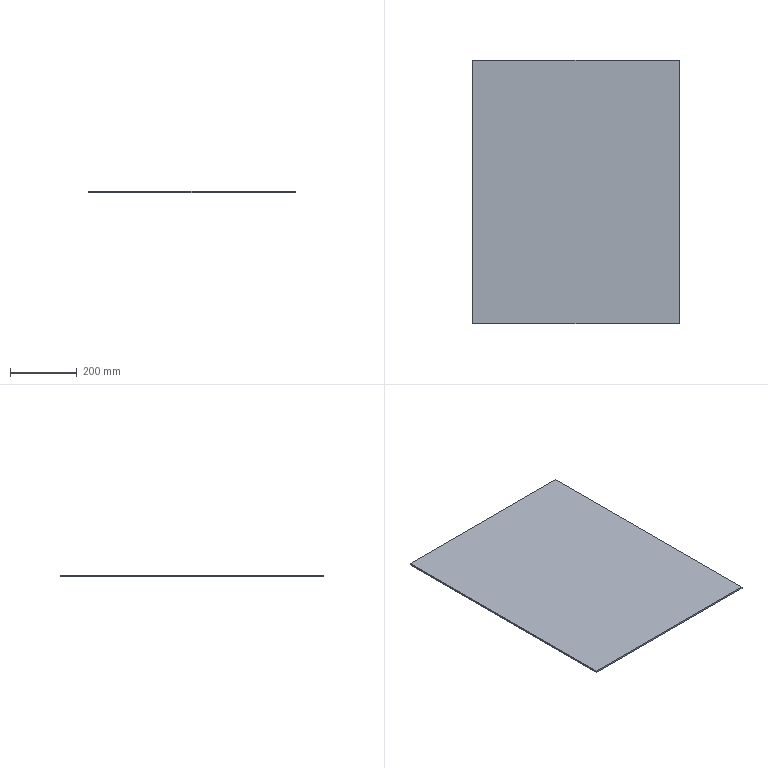Part | SolidWorks | features Extrusion 1 | 1 solid | 6 faces | box 619 x 791 x 5 mm | volume 2448145 mm3 | plane 6
STEP:
#1=CARTESIAN_POINT('',(309.5,-395.5,0.));
#2=VERTEX_POINT('',#1);
#3=CARTESIAN_POINT('',(309.5,395.5,0.));
#4=VERTEX_POINT('',#3);
#5=CARTESIAN_POINT('',(309.5,395.5,0.));
#6=DIRECTION('',(0.,1.,0.));
#7=VECTOR('',#6,1000.);
#8=LINE('',#5,#7);
#9=EDGE_CURVE('',#2,#4,#8,.T.);
#10=ORIENTED_EDGE('',*,*,#9,.T.);
#11=CARTESIAN_POINT('',(309.5,395.5,5.));
#12=VERTEX_POINT('',#11);
#13=CARTESIAN_POINT('',(309.5,395.5,5.));
#14=DIRECTION('',(0.,0.,-1.));
#15=VECTOR('',#14,1000.);
#16=LINE('',#13,#15);
#17=EDGE_CURVE('',#12,#4,#16,.T.);
#18=ORIENTED_EDGE('',*,*,#17,.F.);
#19=CARTESIAN_POINT('',(309.5,-395.5,5.));
#20=VERTEX_POINT('',#19);
#21=CARTESIAN_POINT('',(309.5,395.5,5.));
#22=DIRECTION('',(0.,1.,0.));
#23=VECTOR('',#22,1000.);
#24=LINE('',#21,#23);
#25=EDGE_CURVE('',#20,#12,#24,.T.);
#26=ORIENTED_EDGE('',*,*,#25,.F.);
#27=CARTESIAN_POINT('',(309.5,-395.5,5.));
#28=DIRECTION('',(0.,0.,-1.));
#29=VECTOR('',#28,1000.);
#30=LINE('',#27,#29);
#31=EDGE_CURVE('',#20,#2,#30,.T.);
#32=ORIENTED_EDGE('',*,*,#31,.T.);
#33=EDGE_LOOP('',(#10,#18,#26,#32));
#34=FACE_OUTER_BOUND('',#33,.T.);
#35=CARTESIAN_POINT('',(309.5,395.5,5.));
#36=DIRECTION('',(-1.,0.,0.));
#37=DIRECTION('',(0.,-1.,0.));
#38=AXIS2_PLACEMENT_3D('',#35,#36,#37);
#39=PLANE('',#38);
#40=ADVANCED_FACE('',(#34),#39,.F.);
#41=CARTESIAN_POINT('',(-309.5,395.5,0.));
#42=VERTEX_POINT('',#41);
#43=CARTESIAN_POINT('',(-309.5,395.5,0.));
#44=DIRECTION('',(-1.,0.,0.));
#45=VECTOR('',#44,1000.);
#46=LINE('',#43,#45);
#47=EDGE_CURVE('',#4,#42,#46,.T.);
#48=ORIENTED_EDGE('',*,*,#47,.T.);
#49=CARTESIAN_POINT('',(-309.5,395.5,5.));
#50=VERTEX_POINT('',#49);
#51=CARTESIAN_POINT('',(-309.5,395.5,5.));
#52=DIRECTION('',(0.,0.,-1.));
#53=VECTOR('',#52,1000.);
#54=LINE('',#51,#53);
#55=EDGE_CURVE('',#50,#42,#54,.T.);
#56=ORIENTED_EDGE('',*,*,#55,.F.);
#57=CARTESIAN_POINT('',(-309.5,395.5,5.));
#58=DIRECTION('',(-1.,0.,0.));
#59=VECTOR('',#58,1000.);
#60=LINE('',#57,#59);
#61=EDGE_CURVE('',#12,#50,#60,.T.);
#62=ORIENTED_EDGE('',*,*,#61,.F.);
#63=ORIENTED_EDGE('',*,*,#17,.T.);
#64=EDGE_LOOP('',(#48,#56,#62,#63));
#65=FACE_OUTER_BOUND('',#64,.T.);
#66=CARTESIAN_POINT('',(-309.5,395.5,5.));
#67=DIRECTION('',(0.,-1.,0.));
#68=DIRECTION('',(0.,0.,-1.));
#69=AXIS2_PLACEMENT_3D('',#66,#67,#68);
#70=PLANE('',#69);
#71=ADVANCED_FACE('',(#65),#70,.F.);
#72=CARTESIAN_POINT('',(-309.5,-395.5,0.));
#73=VERTEX_POINT('',#72);
#74=CARTESIAN_POINT('',(-309.5,395.5,0.));
#75=DIRECTION('',(0.,-1.,0.));
#76=VECTOR('',#75,1000.);
#77=LINE('',#74,#76);
#78=EDGE_CURVE('',#42,#73,#77,.T.);
#79=ORIENTED_EDGE('',*,*,#78,.T.);
#80=CARTESIAN_POINT('',(-309.5,-395.5,5.));
#81=VERTEX_POINT('',#80);
#82=CARTESIAN_POINT('',(-309.5,-395.5,5.));
#83=DIRECTION('',(0.,0.,-1.));
#84=VECTOR('',#83,1000.);
#85=LINE('',#82,#84);
#86=EDGE_CURVE('',#81,#73,#85,.T.);
#87=ORIENTED_EDGE('',*,*,#86,.F.);
#88=CARTESIAN_POINT('',(-309.5,395.5,5.));
#89=DIRECTION('',(0.,-1.,0.));
#90=VECTOR('',#89,1000.);
#91=LINE('',#88,#90);
#92=EDGE_CURVE('',#50,#81,#91,.T.);
#93=ORIENTED_EDGE('',*,*,#92,.F.);
#94=ORIENTED_EDGE('',*,*,#55,.T.);
#95=EDGE_LOOP('',(#79,#87,#93,#94));
#96=FACE_OUTER_BOUND('',#95,.T.);
#97=CARTESIAN_POINT('',(-309.5,395.5,5.));
#98=DIRECTION('',(1.,0.,0.));
#99=DIRECTION('',(0.,1.,0.));
#100=AXIS2_PLACEMENT_3D('',#97,#98,#99);
#101=PLANE('',#100);
#102=ADVANCED_FACE('',(#96),#101,.F.);
#103=CARTESIAN_POINT('',(-309.5,-395.5,0.));
#104=DIRECTION('',(1.,0.,0.));
#105=VECTOR('',#104,1000.);
#106=LINE('',#103,#105);
#107=EDGE_CURVE('',#73,#2,#106,.T.);
#108=ORIENTED_EDGE('',*,*,#107,.T.);
#109=ORIENTED_EDGE('',*,*,#31,.F.);
#110=CARTESIAN_POINT('',(-309.5,-395.5,5.));
#111=DIRECTION('',(1.,0.,0.));
#112=VECTOR('',#111,1000.);
#113=LINE('',#110,#112);
#114=EDGE_CURVE('',#81,#20,#113,.T.);
#115=ORIENTED_EDGE('',*,*,#114,.F.);
#116=ORIENTED_EDGE('',*,*,#86,.T.);
#117=EDGE_LOOP('',(#108,#109,#115,#116));
#118=FACE_OUTER_BOUND('',#117,.T.);
#119=CARTESIAN_POINT('',(-309.5,-395.5,5.));
#120=DIRECTION('',(0.,1.,0.));
#121=DIRECTION('',(0.,0.,1.));
#122=AXIS2_PLACEMENT_3D('',#119,#120,#121);
#123=PLANE('',#122);
#124=ADVANCED_FACE('',(#118),#123,.F.);
#125=ORIENTED_EDGE('',*,*,#25,.T.);
#126=ORIENTED_EDGE('',*,*,#61,.T.);
#127=ORIENTED_EDGE('',*,*,#92,.T.);
#128=ORIENTED_EDGE('',*,*,#114,.T.);
#129=EDGE_LOOP('',(#125,#126,#127,#128));
#130=FACE_OUTER_BOUND('',#129,.T.);
#131=CARTESIAN_POINT('',(0.,0.,5.));
#132=DIRECTION('',(0.,0.,1.));
#133=DIRECTION('',(1.,0.,0.));
#134=AXIS2_PLACEMENT_3D('',#131,#132,#133);
#135=PLANE('',#134);
#136=ADVANCED_FACE('',(#130),#135,.T.);
#137=ORIENTED_EDGE('',*,*,#9,.F.);
#138=ORIENTED_EDGE('',*,*,#107,.F.);
#139=ORIENTED_EDGE('',*,*,#78,.F.);
#140=ORIENTED_EDGE('',*,*,#47,.F.);
#141=EDGE_LOOP('',(#137,#138,#139,#140));
#142=FACE_OUTER_BOUND('',#141,.T.);
#143=CARTESIAN_POINT('',(0.,0.,0.));
#144=DIRECTION('',(0.,0.,1.));
#145=DIRECTION('',(1.,0.,0.));
#146=AXIS2_PLACEMENT_3D('',#143,#144,#145);
#147=PLANE('',#146);
#148=ADVANCED_FACE('',(#142),#147,.F.);
#149=CLOSED_SHELL('',(#40,#71,#102,#124,#136,#148));
#150=MANIFOLD_SOLID_BREP('',#149);
#151=CARTESIAN_POINT('',(0.,0.,0.));
#152=DIRECTION('',(0.,0.,1.));
#153=DIRECTION('',(1.,0.,0.));
#154=AXIS2_PLACEMENT_3D('',#151,#152,#153);
#155=(LENGTH_UNIT()NAMED_UNIT(*)SI_UNIT(.MILLI.,.METRE.));
#156=UNCERTAINTY_MEASURE_WITH_UNIT(LENGTH_MEASURE(0.00001),#155,'','');
#157=(NAMED_UNIT(*)PLANE_ANGLE_UNIT()SI_UNIT($,.RADIAN.));
#158=(NAMED_UNIT(*)SI_UNIT($,.STERADIAN.)SOLID_ANGLE_UNIT());
#159=(GEOMETRIC_REPRESENTATION_CONTEXT(3)GLOBAL_UNCERTAINTY_ASSIGNED_CONTEXT((#156))GLOBAL_UNIT_ASSIGNED_CONTEXT((#155,#157,#158))REPRESENTATION_CONTEXT('',''));
#160=ADVANCED_BREP_SHAPE_REPRESENTATION('',(#150,#154),#159);